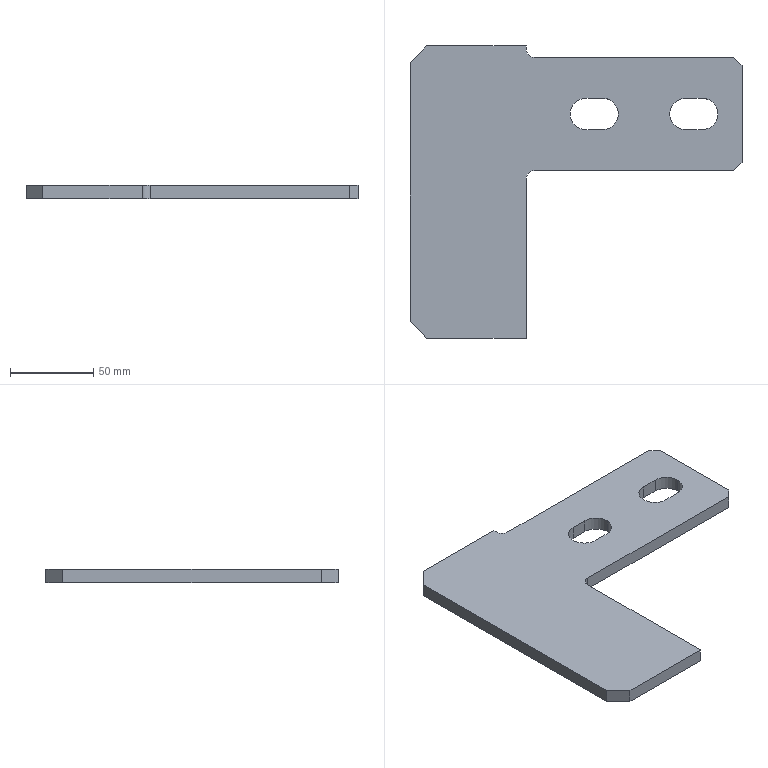Part | STEP file | 筋Plate-194×150-100 | 1 solid | 26 faces | box 200 x 176 x 8 mm | volume 160789 mm3 | plane 18 | cylinder 8 | commonest cylinder face diameters 19 x6 10 x2